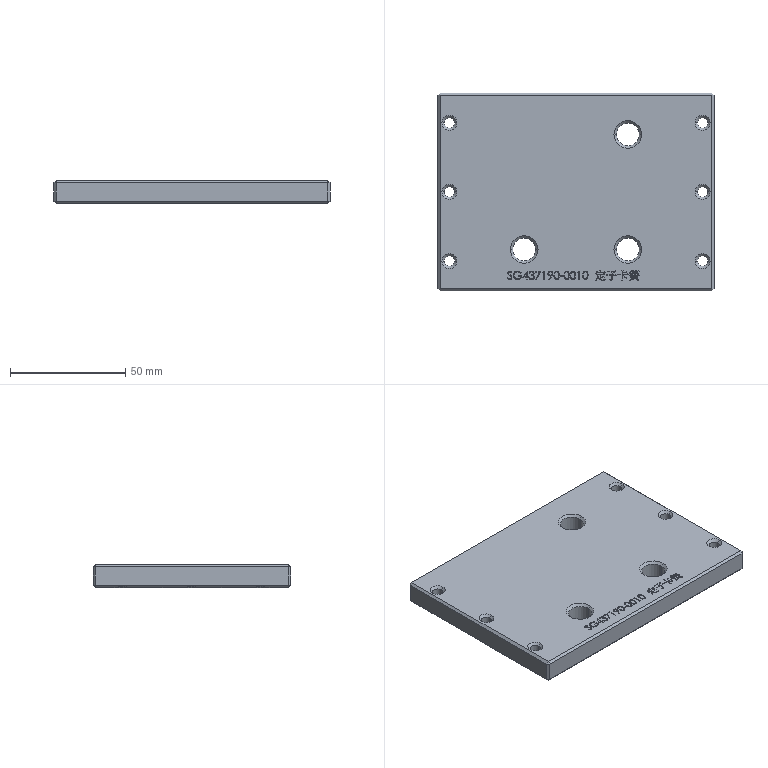Part | STEP file | Base plate-market stator circlip | 1 solid | 446 faces | box 120 x 86 x 10 mm | volume 98205 mm3 | plane 259 | spline 121 | cone 36 | cylinder 30 | commonest cylinder face diameters 4.5 x12 8 x12 10 x6